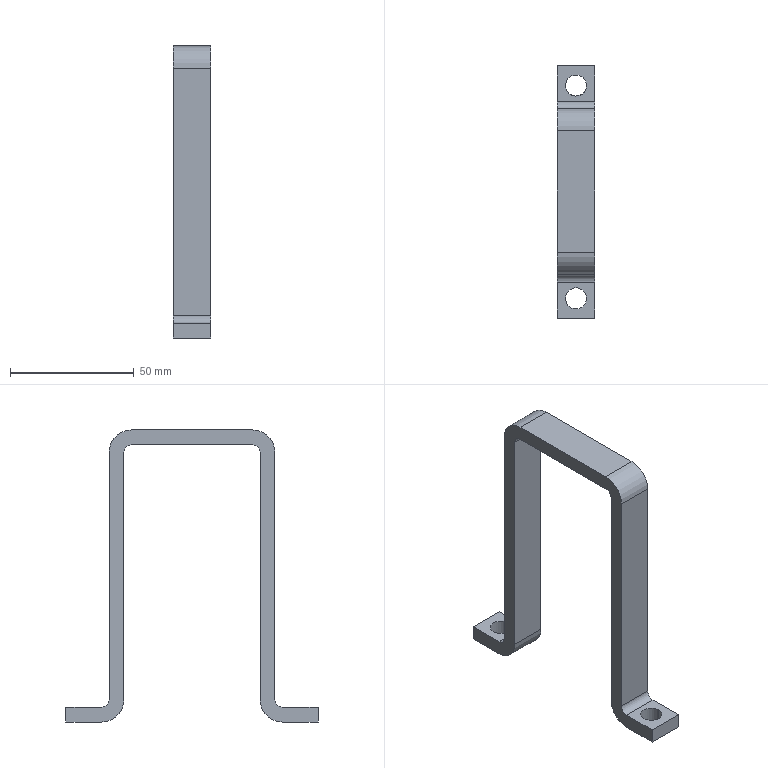Part | STEP file | 1_id726_x_t | 1 solid | 26 faces | box 15 x 102.012 x 118 mm | volume 27733 mm3 | plane 14 | cylinder 12 | commonest cylinder face diameters 6 x4 8.5 x4 18 x4